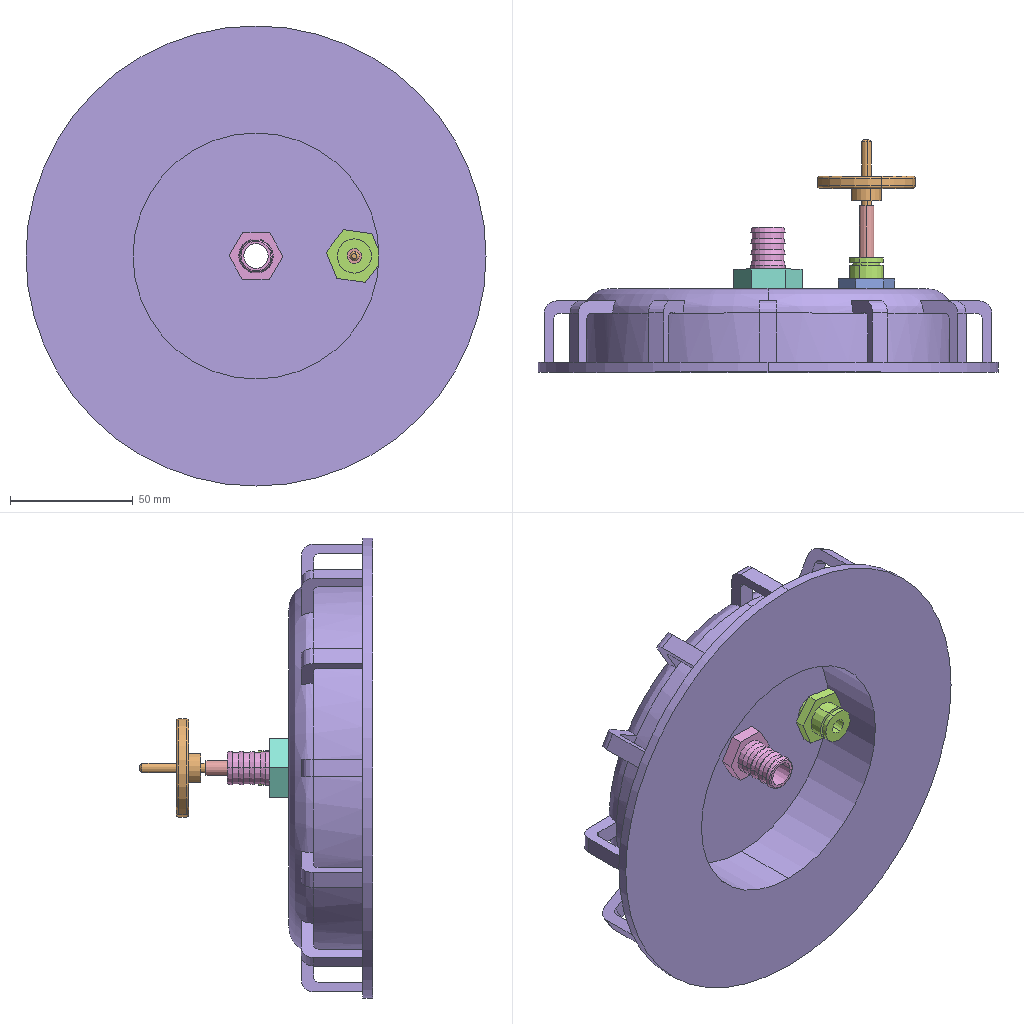Assembly | SolidWorks | 5 different items | 5 placed | box 187 x 95 x 187 mm
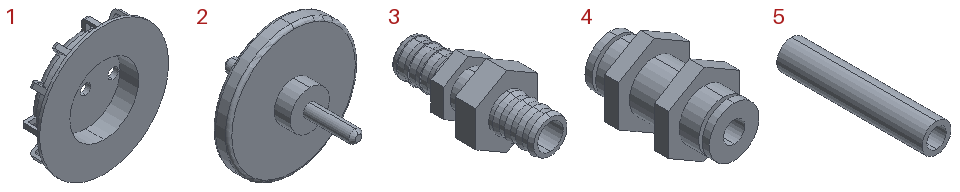Parts list (item | quantity | size | volume | features):
1 | x1 | 187 x 34 x 187 mm | 428914 mm3 | features ICE 4, Fillet 3, CirPattern 1, Cut 1, Extrusion 1
2 | x1 | 40 x 40 x 40 mm | 7162 mm3 | features Chamfer 1, Fillet 1, Revolution 1
3 | x1 | 24 x 55 x 27.713 mm | 7209 mm3 | features ICE 4, Extrusion 1, Fillet 1, RevCut 1
4 | x1 | 20 x 35 x 23.094 mm | 5820 mm3 | features ICE 3, Revolution 1
5 | x1 | 6 x 30 x 6 mm | 471.239 mm3 | features Extrusion 1
Mates (type | each side: item.copy, entity, surface, feature):
Concentric | 1.1 face cylinder Cut-Extrude2 | 4.1 face cylinder Revolve1
Concentric | 1.1 face cylinder Cut-Extrude2 | 3.1 face cylinder Boss-Extrude3
Coincident | 1.1 face plane Boss-Extrude1 | 4.1 face plane Boss-Extrude1
Coincident | 1.1 face plane Cut-Extrude1 | assembly plane
Coincident | 1.1 plane | assembly plane
Concentric | 4.1 face cylinder Cut-Extrude1 | 5.1 face cylinder Boss-Extrude1
Concentric | 5.1 face cylinder Boss-Extrude1 | 2.1 face cylinder Revolve1